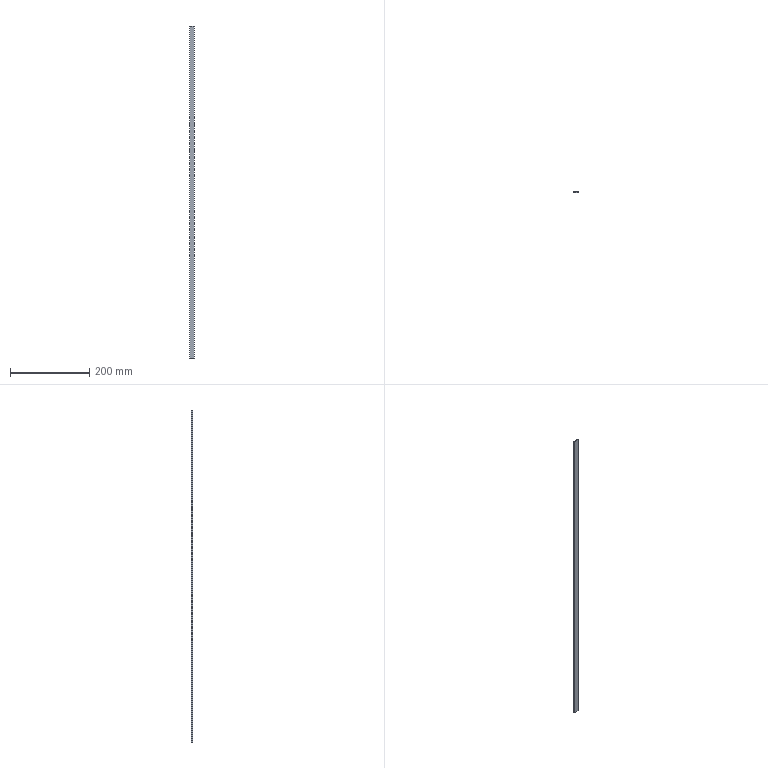Part | SolidWorks | features Extrusion 1, ICE 1 | 1 solid | 10 faces | box 12 x 3 x 840 mm | volume 21840 mm3 | plane 10
STEP:
#1=CARTESIAN_POINT('',(-31.901,24.125,0.));
#2=VERTEX_POINT('',#1);
#3=CARTESIAN_POINT('',(-31.901,21.125,0.));
#4=VERTEX_POINT('',#3);
#5=CARTESIAN_POINT('',(-31.901,21.125,0.));
#6=DIRECTION('',(0.,-1.,0.));
#7=VECTOR('',#6,1000.);
#8=LINE('',#5,#7);
#9=EDGE_CURVE('',#2,#4,#8,.T.);
#10=ORIENTED_EDGE('',*,*,#9,.T.);
#11=CARTESIAN_POINT('',(-31.901,21.125,840.));
#12=VERTEX_POINT('',#11);
#13=CARTESIAN_POINT('',(-31.901,21.125,840.));
#14=DIRECTION('',(0.,0.,-1.));
#15=VECTOR('',#14,1000.);
#16=LINE('',#13,#15);
#17=EDGE_CURVE('',#12,#4,#16,.T.);
#18=ORIENTED_EDGE('',*,*,#17,.F.);
#19=CARTESIAN_POINT('',(-31.901,24.125,840.));
#20=VERTEX_POINT('',#19);
#21=CARTESIAN_POINT('',(-31.901,21.125,840.));
#22=DIRECTION('',(0.,-1.,0.));
#23=VECTOR('',#22,1000.);
#24=LINE('',#21,#23);
#25=EDGE_CURVE('',#20,#12,#24,.T.);
#26=ORIENTED_EDGE('',*,*,#25,.F.);
#27=CARTESIAN_POINT('',(-31.901,24.125,840.));
#28=DIRECTION('',(0.,0.,-1.));
#29=VECTOR('',#28,1000.);
#30=LINE('',#27,#29);
#31=EDGE_CURVE('',#20,#2,#30,.T.);
#32=ORIENTED_EDGE('',*,*,#31,.T.);
#33=EDGE_LOOP('',(#10,#18,#26,#32));
#34=FACE_OUTER_BOUND('',#33,.T.);
#35=CARTESIAN_POINT('',(-31.901,21.125,840.));
#36=DIRECTION('',(1.,0.,0.));
#37=DIRECTION('',(0.,0.,-1.));
#38=AXIS2_PLACEMENT_3D('',#35,#36,#37);
#39=PLANE('',#38);
#40=ADVANCED_FACE('',(#34),#39,.F.);
#41=CARTESIAN_POINT('',(-19.901,21.125,0.));
#42=VERTEX_POINT('',#41);
#43=CARTESIAN_POINT('',(-19.901,21.125,0.));
#44=DIRECTION('',(1.,0.,0.));
#45=VECTOR('',#44,1000.);
#46=LINE('',#43,#45);
#47=EDGE_CURVE('',#4,#42,#46,.T.);
#48=ORIENTED_EDGE('',*,*,#47,.T.);
#49=CARTESIAN_POINT('',(-19.901,21.125,840.));
#50=VERTEX_POINT('',#49);
#51=CARTESIAN_POINT('',(-19.901,21.125,840.));
#52=DIRECTION('',(0.,0.,-1.));
#53=VECTOR('',#52,1000.);
#54=LINE('',#51,#53);
#55=EDGE_CURVE('',#50,#42,#54,.T.);
#56=ORIENTED_EDGE('',*,*,#55,.F.);
#57=CARTESIAN_POINT('',(-19.901,21.125,840.));
#58=DIRECTION('',(1.,0.,0.));
#59=VECTOR('',#58,1000.);
#60=LINE('',#57,#59);
#61=EDGE_CURVE('',#12,#50,#60,.T.);
#62=ORIENTED_EDGE('',*,*,#61,.F.);
#63=ORIENTED_EDGE('',*,*,#17,.T.);
#64=EDGE_LOOP('',(#48,#56,#62,#63));
#65=FACE_OUTER_BOUND('',#64,.T.);
#66=CARTESIAN_POINT('',(-19.901,21.125,840.));
#67=DIRECTION('',(0.,1.,0.));
#68=DIRECTION('',(0.,0.,1.));
#69=AXIS2_PLACEMENT_3D('',#66,#67,#68);
#70=PLANE('',#69);
#71=ADVANCED_FACE('',(#65),#70,.F.);
#72=CARTESIAN_POINT('',(-19.901,24.125,0.));
#73=VERTEX_POINT('',#72);
#74=CARTESIAN_POINT('',(-19.901,24.125,0.));
#75=DIRECTION('',(0.,1.,0.));
#76=VECTOR('',#75,1000.);
#77=LINE('',#74,#76);
#78=EDGE_CURVE('',#42,#73,#77,.T.);
#79=ORIENTED_EDGE('',*,*,#78,.T.);
#80=CARTESIAN_POINT('',(-19.901,24.125,840.));
#81=VERTEX_POINT('',#80);
#82=CARTESIAN_POINT('',(-19.901,24.125,840.));
#83=DIRECTION('',(0.,0.,-1.));
#84=VECTOR('',#83,1000.);
#85=LINE('',#82,#84);
#86=EDGE_CURVE('',#81,#73,#85,.T.);
#87=ORIENTED_EDGE('',*,*,#86,.F.);
#88=CARTESIAN_POINT('',(-19.901,24.125,840.));
#89=DIRECTION('',(0.,1.,0.));
#90=VECTOR('',#89,1000.);
#91=LINE('',#88,#90);
#92=EDGE_CURVE('',#50,#81,#91,.T.);
#93=ORIENTED_EDGE('',*,*,#92,.F.);
#94=ORIENTED_EDGE('',*,*,#55,.T.);
#95=EDGE_LOOP('',(#79,#87,#93,#94));
#96=FACE_OUTER_BOUND('',#95,.T.);
#97=CARTESIAN_POINT('',(-19.901,24.125,840.));
#98=DIRECTION('',(-1.,0.,0.));
#99=DIRECTION('',(0.,0.,1.));
#100=AXIS2_PLACEMENT_3D('',#97,#98,#99);
#101=PLANE('',#100);
#102=ADVANCED_FACE('',(#96),#101,.F.);
#103=CARTESIAN_POINT('',(-31.901,24.125,0.));
#104=DIRECTION('',(-1.,0.,0.));
#105=VECTOR('',#104,1000.);
#106=LINE('',#103,#105);
#107=EDGE_CURVE('',#73,#2,#106,.T.);
#108=ORIENTED_EDGE('',*,*,#107,.T.);
#109=ORIENTED_EDGE('',*,*,#31,.F.);
#110=CARTESIAN_POINT('',(-31.901,24.125,840.));
#111=DIRECTION('',(-1.,0.,0.));
#112=VECTOR('',#111,1000.);
#113=LINE('',#110,#112);
#114=EDGE_CURVE('',#81,#20,#113,.T.);
#115=ORIENTED_EDGE('',*,*,#114,.F.);
#116=ORIENTED_EDGE('',*,*,#86,.T.);
#117=EDGE_LOOP('',(#108,#109,#115,#116));
#118=FACE_OUTER_BOUND('',#117,.T.);
#119=CARTESIAN_POINT('',(-31.901,24.125,840.));
#120=DIRECTION('',(0.,-1.,0.));
#121=DIRECTION('',(0.,0.,-1.));
#122=AXIS2_PLACEMENT_3D('',#119,#120,#121);
#123=PLANE('',#122);
#124=ADVANCED_FACE('',(#118),#123,.F.);
#125=CARTESIAN_POINT('',(-30.901,22.125,840.));
#126=VERTEX_POINT('',#125);
#127=CARTESIAN_POINT('',(-20.901,22.125,840.));
#128=VERTEX_POINT('',#127);
#129=CARTESIAN_POINT('',(-20.901,22.125,840.));
#130=DIRECTION('',(1.,0.,0.));
#131=VECTOR('',#130,1000.);
#132=LINE('',#129,#131);
#133=EDGE_CURVE('',#126,#128,#132,.T.);
#134=ORIENTED_EDGE('',*,*,#133,.F.);
#135=CARTESIAN_POINT('',(-30.901,23.125,840.));
#136=VERTEX_POINT('',#135);
#137=CARTESIAN_POINT('',(-30.901,22.125,840.));
#138=DIRECTION('',(0.,-1.,0.));
#139=VECTOR('',#138,1000.);
#140=LINE('',#137,#139);
#141=EDGE_CURVE('',#136,#126,#140,.T.);
#142=ORIENTED_EDGE('',*,*,#141,.F.);
#143=CARTESIAN_POINT('',(-20.901,23.125,840.));
#144=VERTEX_POINT('',#143);
#145=CARTESIAN_POINT('',(-30.901,23.125,840.));
#146=DIRECTION('',(-1.,0.,0.));
#147=VECTOR('',#146,1000.);
#148=LINE('',#145,#147);
#149=EDGE_CURVE('',#144,#136,#148,.T.);
#150=ORIENTED_EDGE('',*,*,#149,.F.);
#151=CARTESIAN_POINT('',(-20.901,23.125,840.));
#152=DIRECTION('',(0.,1.,0.));
#153=VECTOR('',#152,1000.);
#154=LINE('',#151,#153);
#155=EDGE_CURVE('',#128,#144,#154,.T.);
#156=ORIENTED_EDGE('',*,*,#155,.F.);
#157=EDGE_LOOP('',(#134,#142,#150,#156));
#158=FACE_BOUND('',#157,.T.);
#159=ORIENTED_EDGE('',*,*,#25,.T.);
#160=ORIENTED_EDGE('',*,*,#61,.T.);
#161=ORIENTED_EDGE('',*,*,#92,.T.);
#162=ORIENTED_EDGE('',*,*,#114,.T.);
#163=EDGE_LOOP('',(#159,#160,#161,#162));
#164=FACE_OUTER_BOUND('',#163,.T.);
#165=CARTESIAN_POINT('',(0.,0.,840.));
#166=DIRECTION('',(0.,0.,-1.));
#167=DIRECTION('',(-1.,0.,0.));
#168=AXIS2_PLACEMENT_3D('',#165,#166,#167);
#169=PLANE('',#168);
#170=ADVANCED_FACE('',(#158,#164),#169,.F.);
#171=CARTESIAN_POINT('',(-30.901,23.125,0.));
#172=VERTEX_POINT('',#171);
#173=CARTESIAN_POINT('',(-30.901,22.125,0.));
#174=VERTEX_POINT('',#173);
#175=CARTESIAN_POINT('',(-30.901,22.125,0.));
#176=DIRECTION('',(0.,-1.,0.));
#177=VECTOR('',#176,1000.);
#178=LINE('',#175,#177);
#179=EDGE_CURVE('',#172,#174,#178,.T.);
#180=ORIENTED_EDGE('',*,*,#179,.T.);
#181=CARTESIAN_POINT('',(-20.901,22.125,0.));
#182=VERTEX_POINT('',#181);
#183=CARTESIAN_POINT('',(-20.901,22.125,0.));
#184=DIRECTION('',(1.,0.,0.));
#185=VECTOR('',#184,1000.);
#186=LINE('',#183,#185);
#187=EDGE_CURVE('',#174,#182,#186,.T.);
#188=ORIENTED_EDGE('',*,*,#187,.T.);
#189=CARTESIAN_POINT('',(-20.901,23.125,0.));
#190=VERTEX_POINT('',#189);
#191=CARTESIAN_POINT('',(-20.901,23.125,0.));
#192=DIRECTION('',(0.,1.,0.));
#193=VECTOR('',#192,1000.);
#194=LINE('',#191,#193);
#195=EDGE_CURVE('',#182,#190,#194,.T.);
#196=ORIENTED_EDGE('',*,*,#195,.T.);
#197=CARTESIAN_POINT('',(-30.901,23.125,0.));
#198=DIRECTION('',(-1.,0.,0.));
#199=VECTOR('',#198,1000.);
#200=LINE('',#197,#199);
#201=EDGE_CURVE('',#190,#172,#200,.T.);
#202=ORIENTED_EDGE('',*,*,#201,.T.);
#203=EDGE_LOOP('',(#180,#188,#196,#202));
#204=FACE_BOUND('',#203,.T.);
#205=ORIENTED_EDGE('',*,*,#9,.F.);
#206=ORIENTED_EDGE('',*,*,#107,.F.);
#207=ORIENTED_EDGE('',*,*,#78,.F.);
#208=ORIENTED_EDGE('',*,*,#47,.F.);
#209=EDGE_LOOP('',(#205,#206,#207,#208));
#210=FACE_OUTER_BOUND('',#209,.T.);
#211=CARTESIAN_POINT('',(0.,0.,0.));
#212=DIRECTION('',(0.,0.,-1.));
#213=DIRECTION('',(-1.,0.,0.));
#214=AXIS2_PLACEMENT_3D('',#211,#212,#213);
#215=PLANE('',#214);
#216=ADVANCED_FACE('',(#204,#210),#215,.T.);
#217=ORIENTED_EDGE('',*,*,#141,.T.);
#218=CARTESIAN_POINT('',(-30.901,22.125,0.));
#219=DIRECTION('',(0.,0.,1.));
#220=VECTOR('',#219,1000.);
#221=LINE('',#218,#220);
#222=EDGE_CURVE('',#174,#126,#221,.T.);
#223=ORIENTED_EDGE('',*,*,#222,.F.);
#224=ORIENTED_EDGE('',*,*,#179,.F.);
#225=CARTESIAN_POINT('',(-30.901,23.125,0.));
#226=DIRECTION('',(0.,0.,1.));
#227=VECTOR('',#226,1000.);
#228=LINE('',#225,#227);
#229=EDGE_CURVE('',#172,#136,#228,.T.);
#230=ORIENTED_EDGE('',*,*,#229,.T.);
#231=EDGE_LOOP('',(#217,#223,#224,#230));
#232=FACE_OUTER_BOUND('',#231,.T.);
#233=CARTESIAN_POINT('',(-30.901,22.125,0.));
#234=DIRECTION('',(-1.,0.,0.));
#235=DIRECTION('',(0.,0.,1.));
#236=AXIS2_PLACEMENT_3D('',#233,#234,#235);
#237=PLANE('',#236);
#238=ADVANCED_FACE('',(#232),#237,.F.);
#239=ORIENTED_EDGE('',*,*,#149,.T.);
#240=ORIENTED_EDGE('',*,*,#229,.F.);
#241=ORIENTED_EDGE('',*,*,#201,.F.);
#242=CARTESIAN_POINT('',(-20.901,23.125,0.));
#243=DIRECTION('',(0.,0.,1.));
#244=VECTOR('',#243,1000.);
#245=LINE('',#242,#244);
#246=EDGE_CURVE('',#190,#144,#245,.T.);
#247=ORIENTED_EDGE('',*,*,#246,.T.);
#248=EDGE_LOOP('',(#239,#240,#241,#247));
#249=FACE_OUTER_BOUND('',#248,.T.);
#250=CARTESIAN_POINT('',(-30.901,23.125,0.));
#251=DIRECTION('',(0.,1.,0.));
#252=DIRECTION('',(0.,0.,1.));
#253=AXIS2_PLACEMENT_3D('',#250,#251,#252);
#254=PLANE('',#253);
#255=ADVANCED_FACE('',(#249),#254,.F.);
#256=ORIENTED_EDGE('',*,*,#155,.T.);
#257=ORIENTED_EDGE('',*,*,#246,.F.);
#258=ORIENTED_EDGE('',*,*,#195,.F.);
#259=CARTESIAN_POINT('',(-20.901,22.125,0.));
#260=DIRECTION('',(0.,0.,1.));
#261=VECTOR('',#260,1000.);
#262=LINE('',#259,#261);
#263=EDGE_CURVE('',#182,#128,#262,.T.);
#264=ORIENTED_EDGE('',*,*,#263,.T.);
#265=EDGE_LOOP('',(#256,#257,#258,#264));
#266=FACE_OUTER_BOUND('',#265,.T.);
#267=CARTESIAN_POINT('',(-20.901,23.125,0.));
#268=DIRECTION('',(1.,0.,0.));
#269=DIRECTION('',(0.,0.,-1.));
#270=AXIS2_PLACEMENT_3D('',#267,#268,#269);
#271=PLANE('',#270);
#272=ADVANCED_FACE('',(#266),#271,.F.);
#273=ORIENTED_EDGE('',*,*,#133,.T.);
#274=ORIENTED_EDGE('',*,*,#263,.F.);
#275=ORIENTED_EDGE('',*,*,#187,.F.);
#276=ORIENTED_EDGE('',*,*,#222,.T.);
#277=EDGE_LOOP('',(#273,#274,#275,#276));
#278=FACE_OUTER_BOUND('',#277,.T.);
#279=CARTESIAN_POINT('',(-20.901,22.125,0.));
#280=DIRECTION('',(0.,-1.,0.));
#281=DIRECTION('',(0.,0.,-1.));
#282=AXIS2_PLACEMENT_3D('',#279,#280,#281);
#283=PLANE('',#282);
#284=ADVANCED_FACE('',(#278),#283,.F.);
#285=CLOSED_SHELL('',(#40,#71,#102,#124,#170,#216,#238,#255,#272,#284));
#286=MANIFOLD_SOLID_BREP('',#285);
#287=CARTESIAN_POINT('',(0.,0.,0.));
#288=DIRECTION('',(0.,0.,1.));
#289=DIRECTION('',(1.,0.,0.));
#290=AXIS2_PLACEMENT_3D('',#287,#288,#289);
#291=(LENGTH_UNIT()NAMED_UNIT(*)SI_UNIT(.MILLI.,.METRE.));
#292=UNCERTAINTY_MEASURE_WITH_UNIT(LENGTH_MEASURE(0.00001),#291,'','');
#293=(NAMED_UNIT(*)PLANE_ANGLE_UNIT()SI_UNIT($,.RADIAN.));
#294=(NAMED_UNIT(*)SI_UNIT($,.STERADIAN.)SOLID_ANGLE_UNIT());
#295=(GEOMETRIC_REPRESENTATION_CONTEXT(3)GLOBAL_UNCERTAINTY_ASSIGNED_CONTEXT((#292))GLOBAL_UNIT_ASSIGNED_CONTEXT((#291,#293,#294))REPRESENTATION_CONTEXT('',''));
#296=ADVANCED_BREP_SHAPE_REPRESENTATION('',(#286,#290),#295);